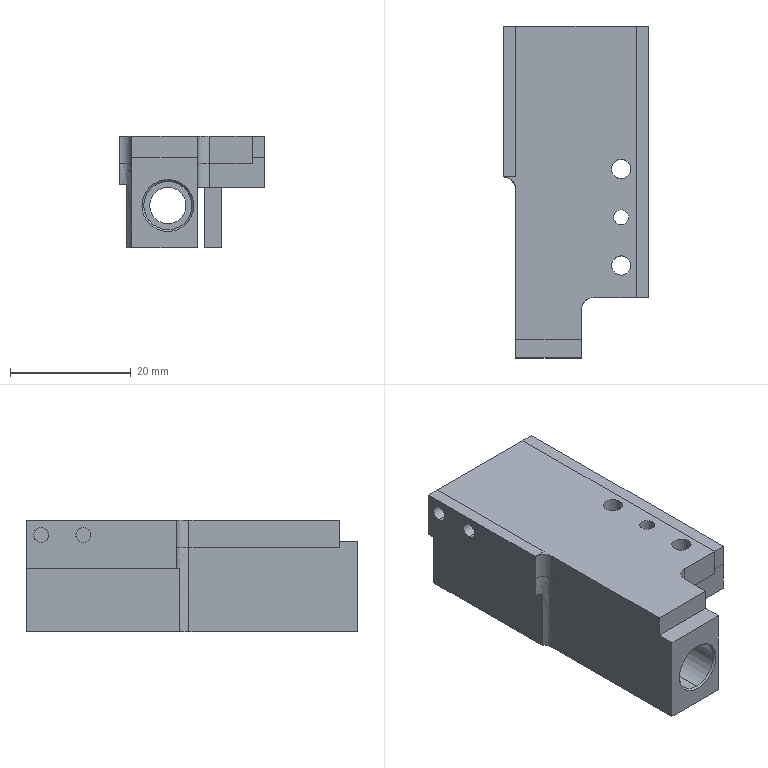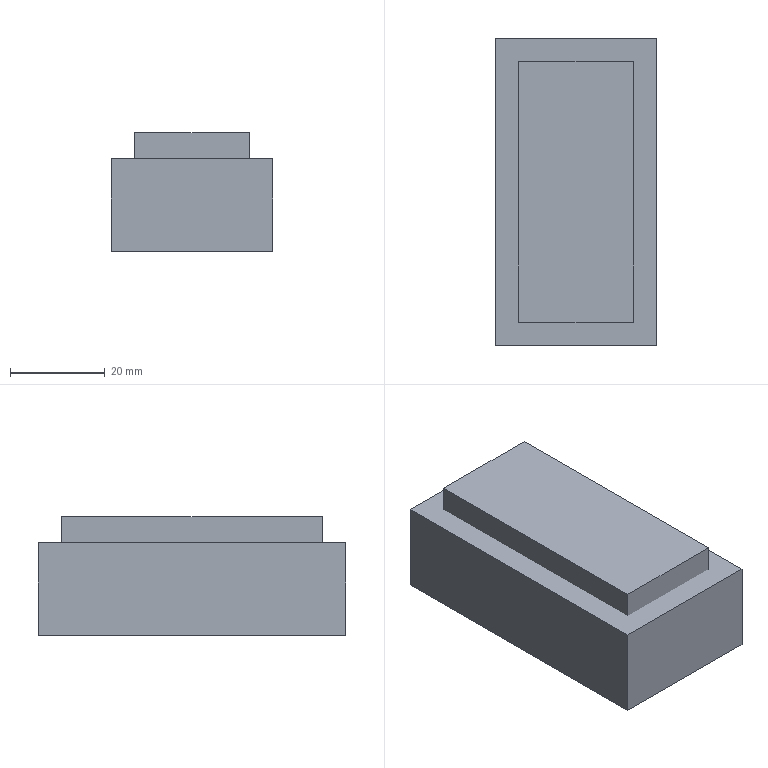CAM job | NX | 3+2 milling, drilling | part box 24.15 x 55 x 18.5 mm | stock box 34.15 x 65 x 25 mm
Tools:
number,name,description,diameter,corner_radius,flute_length,length,flutes
1,D63,Milling Tool-5 Parameters,63.0,0.0,50.0,75.0,2
7,D6A45,Milling Tool-5 Parameters,6.0,0.0,50.0,75.0,2
12,2.5ZT,Drilling Tool,2.5,0.0,35.0,50.0,2
13,3.2ZT,Drilling Tool,3.2,0.0,35.0,50.0,2
10,D10,Milling Tool-5 Parameters,10.0,0.0,50.0,75.0,2
2,D2,Milling Tool-5 Parameters,2.0,0.0,50.0,75.0,2
6,D6,Milling Tool-5 Parameters,6.0,0.0,50.0,75.0,2
4,D4,Milling Tool-5 Parameters,4.0,0.0,50.0,75.0,2
3,D3,Milling Tool-5 Parameters,3.0,0.0,50.0,75.0,2
15,5.5ZT,Drilling Tool,5.5,0.0,35.0,50.0,2
Operations:
program,operation,operation_type,tool,method,geometry_group,spindle_rpm,surface_speed,feed_per_tooth,feed_cut,feed_plunge,cut_length_mm,path_length_mm,cut_time_min,machine_time_min
1,FLOOR_WALL,VolumeBased25DMillingOperation,D63,METHOD,A,6500.0,1286.0,0.1154,1500.0,100.0,140.0,194.0,0.0933,0.0987
1,DRILLING,Operation,D6A45,METHOD,A,5000.0,94.0,0.025,250.0,0.0,12.0,114.823,0.048,0.0583
1,DRILLING_COPY,Operation,2.5ZT,METHOD,A,2000.0,15.0,0.03,120.0,0.0,13.251,86.502,0.1104,0.1178
1,DRILLING_COPY_COPY,Operation,3.2ZT,METHOD,A,2000.0,15.0,0.03,120.0,0.0,26.923,133.124,0.2244,0.235
1,ADAPTIVE_MILLING,CavityMilling,D10,METHOD,A,9500.0,298.0,0.1579,3000.0,1000.0,1551.65,1642.65,0.5192,0.5283
1,ZLEVEL_PROFILE,ZLevelMilling,D10,METHOD,A,9500.0,298.0,0.0789,1500.0,100.0,194.508,288.508,0.1297,0.1391
1,FLOOR_WALL_1_COPY_1,VolumeBased25DMillingOperation,D10,METHOD,A,9500.0,298.0,0.1579,3000.0,1000.0,95.721,229.318,0.0359,0.0493
1,FLOOR_WALL_1_COPY,VolumeBased25DMillingOperation,D10,METHOD,A,9500.0,298.0,0.0789,1500.0,1000.0,70.691,137.691,0.0479,0.0546
1,ZLEVEL_PROFILE_COPY,ZLevelMilling,D2,METHOD,A,7000.0,43.0,0.0571,800.0,100.0,679.359,1122.854,0.8492,0.8935
1,ZLEVEL_PROFILE_COPY_COPY,ZLevelMilling,D2,METHOD,A,7000.0,43.0,0.0571,800.0,100.0,529.437,894.267,0.6618,0.6983
2,FLOOR_WALL_COPY,VolumeBased25DMillingOperation,D63,METHOD,B,6500.0,1286.0,0.1154,1500.0,100.0,938.0,2045.002,0.6253,0.736
2,FLOOR_WALL_1,VolumeBased25DMillingOperation,D10,METHOD,B,9500.0,298.0,0.1579,3000.0,1000.0,1863.816,2625.451,0.6321,0.7083
2,CAVITY_MILL,CavityMilling,D10,METHOD,B,9500.0,298.0,0.1579,3000.0,1000.0,637.273,718.072,0.2774,0.2855
2,CAVITY_MILL_COPY,CavityMilling,D6,METHOD,B,9500.0,179.0,0.1053,2000.0,1000.0,1222.12,1955.02,0.8032,0.8765
2,FLOOR_WALL_1_COPY_COPY,VolumeBased25DMillingOperation,D6,METHOD,B,9500.0,298.0,0.0789,1500.0,1000.0,466.249,784.726,0.3133,0.3452
2,HOLE_MILLING,CylinderMilling,D4,METHOD,B,9500.0,119.0,0.0789,1500.0,100.0,121.863,300.863,0.0812,0.0991
2,CAVITY_MILL_COPY_COPY,CavityMilling,D3,METHOD,B,9500.0,89.0,0.0632,1200.0,1000.0,868.604,1332.059,0.7404,0.7867
2,PLANAR_MILL,PlanarMilling,D6A45,METHOD,B,9500.0,179.0,0.0658,1250.0,100.0,193.795,336.029,0.155,0.1693
2,PLANAR_MILL_COPY,PlanarMilling,D6A45,METHOD,B,9500.0,179.0,0.0658,1250.0,100.0,159.143,581.224,0.1273,0.1695
3,DRILLING_COPY_1,Operation,D6A45,METHOD,C,5000.0,94.0,0.025,250.0,0.0,9.2,103.366,0.0368,0.0462
3,DRILLING_COPY_COPY_1,Operation,2.5ZT,METHOD,C,2000.0,15.0,0.03,120.0,0.0,16.302,117.57,0.1359,0.146
4,DRILLING_COPY_1_COPY,Operation,D6A45,METHOD,D,5000.0,94.0,0.025,250.0,0.0,9.2,89.016,0.0368,0.0448
4,DRILLING_COPY_COPY_1_COPY,Operation,2.5ZT,METHOD,D,2000.0,15.0,0.03,120.0,0.0,14.502,99.62,0.1209,0.1294
5,DRILLING_COPY_1_COPY_COPY,Operation,D6A45,METHOD,E,5000.0,94.0,0.025,250.0,0.0,4.6,69.2,0.0184,0.0249
5,DRILLING_COPY_1_COPY_COPY_COPY,Operation,5.5ZT,METHOD,E,1500.0,25.0,0.04,120.0,0.0,40.152,140.305,0.3346,0.3446
5,HOLE_MILLING_1,CylinderMilling,D6,METHOD,E,9500.0,179.0,0.0789,1500.0,100.0,160.171,229.468,0.1068,0.1137
5,HOLE_MILLING_1_COPY,CylinderMilling,D4,METHOD,E,9500.0,179.0,0.0789,1500.0,100.0,221.07,314.07,0.1474,0.1567
5,PLANAR_MILL_COPY_COPY,PlanarMilling,D6A45,METHOD,E,9500.0,179.0,0.0658,1250.0,100.0,30.36,86.36,0.0243,0.0299
5,刀补6,CylinderMilling,D6,METHOD,E,9500.0,179.0,0.0632,1200.0,100.0,42.663,111.96,0.0356,0.0425
5,刀补4,CylinderMilling,D4,METHOD,E,9500.0,179.0,0.0632,1200.0,100.0,56.188,149.188,0.0468,0.0561
6,刀补,CylinderMilling,D6,METHOD,F,9500.0,179.0,0.0632,1200.0,100.0,169.005,280.305,0.1408,0.152
7,FLOOR_WALL_1_COPY_1_COPY,VolumeBased25DMillingOperation,D10,METHOD,G,9500.0,298.0,0.1579,3000.0,1000.0,2043.677,2431.76,0.6879,0.7267
7,FLOOR_WALL_1_COPY_COPY_1,VolumeBased25DMillingOperation,D6,METHOD,G,9500.0,298.0,0.0789,1500.0,1000.0,557.192,746.235,0.3738,0.3927
7,PLANAR_MILL_COPY_1,PlanarMilling,D6A45,METHOD,G,9500.0,179.0,0.0658,1250.0,100.0,67.864,123.864,0.0543,0.0599
7,PLANAR_MILL_COPY_1_COPY,PlanarMilling,D6A45,METHOD,G,9500.0,179.0,0.0658,1250.0,100.0,144.352,305.447,0.1155,0.1316
7,PLANAR_MILL_COPY_1_COPY_1,PlanarMilling,D6A45,METHOD,G,9500.0,179.0,0.0658,1250.0,100.0,73.001,316.542,0.0584,0.0828